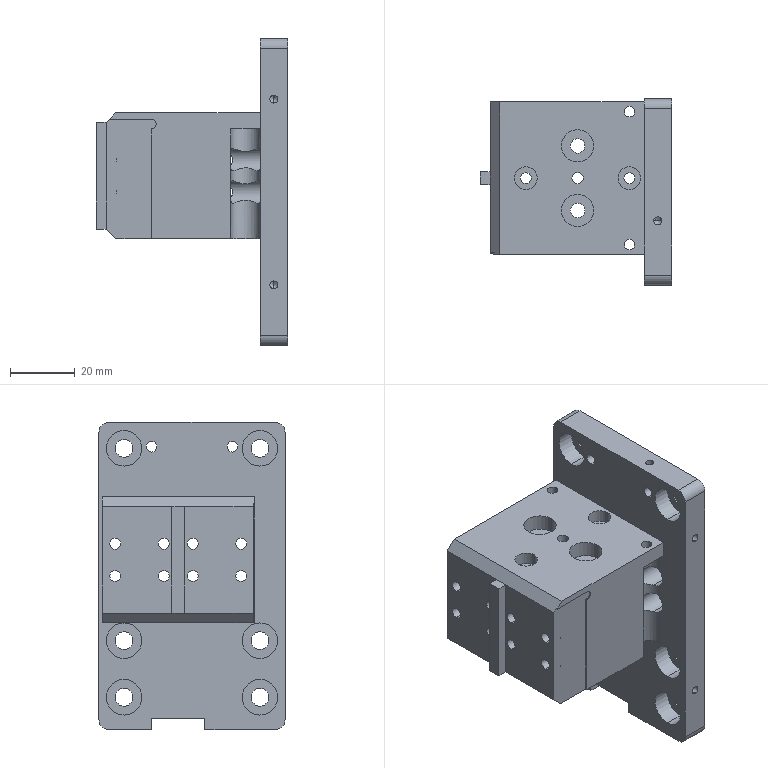Part | STEP file | 1 solid | 204 faces | box 59.1 x 57.6 x 95 mm | volume 75774 mm3 | cylinder 129 | plane 49 | cone 26 | commonest cylinder face diameters 7 x36 3.4 x20 2.5 x16 5.5 x12 11 x12 3.3 x10